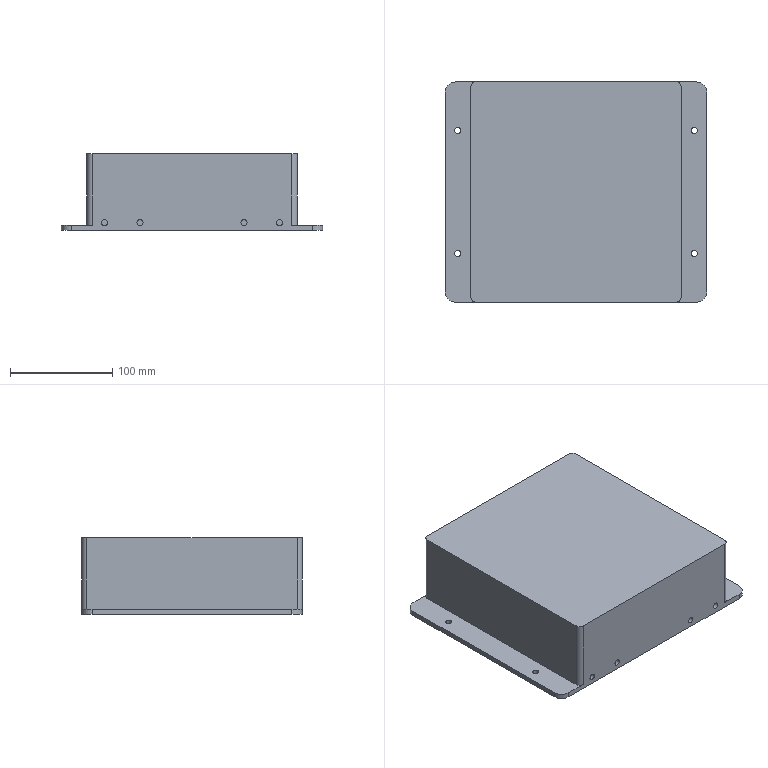NC program | NX | posted with a generic post | part box 255 x 215 x 75 mm
Whole program:
N10 G17 G21 G94 G90
(DRILLING_COPY_1 , TOOL : D6A45)
N12 T01 M6
N14 G54
N16 G17 G0 G90 X85.25 Y29.85 B0. C0. S5000 M3
N18 G43 Z30. H1
N20 G94 G81 G98 Z-1. F350. R3.
N22 X50.75
N24 X-50.75
N26 X-85.25
N28 G80
N30 G0 X-85.25 Y29.85 Z30.
N32 M5
(DRILLING_COPY_COPY , TOOL : 6.0ZT)
N34 T16 M6
N36 G54
N38 G17 G0 G90 X85.25 Y29.85 B0. C0. S2000 M3
N40 G43 Z30. H16
N42 G94 G83 G98 Z-8.303 F250. Q2. R3.
N44 X50.75
N46 X-50.75
N48 X-85.25
N50 G80
N52 G0 X-85.25 Y29.85 Z30.
N54 M5
N56 M2